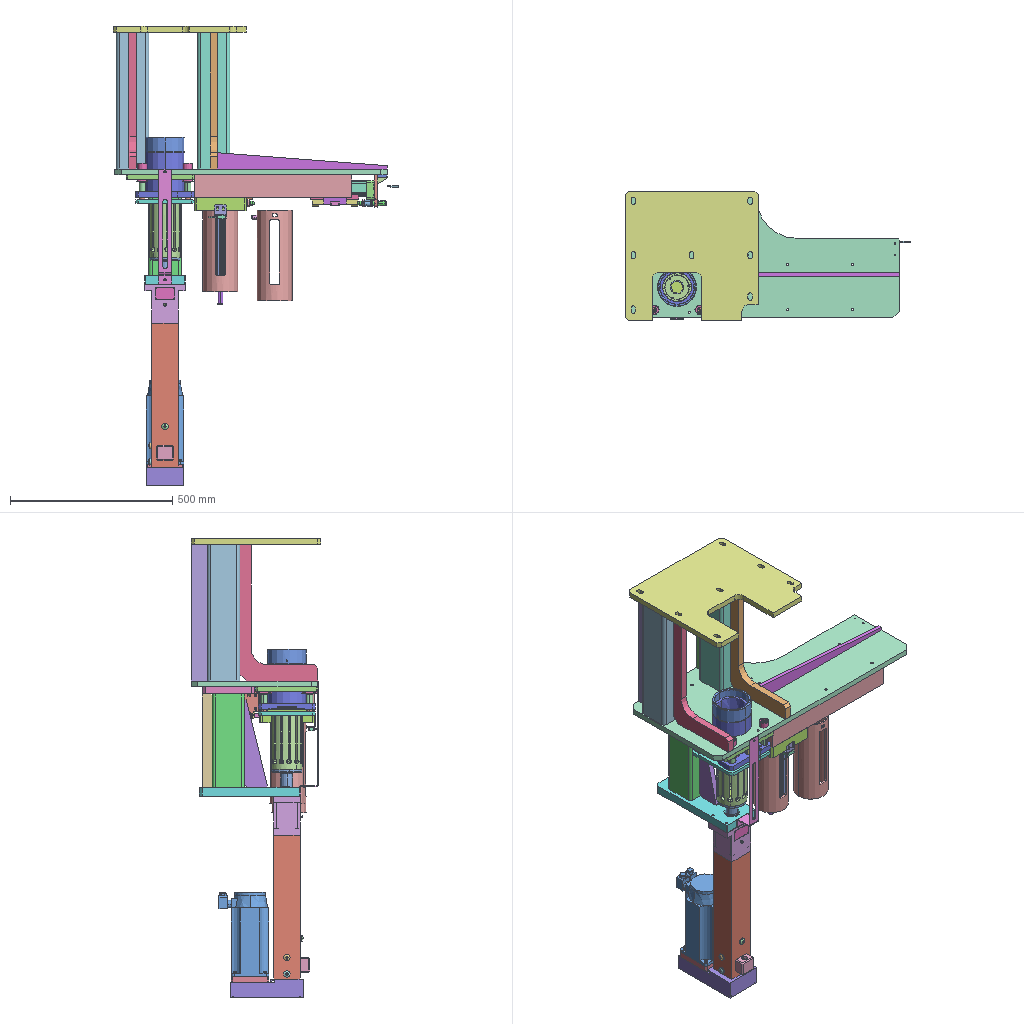Assembly | STEP file | 44 different items | 185 placed | box 880 x 400 x 1414 mm
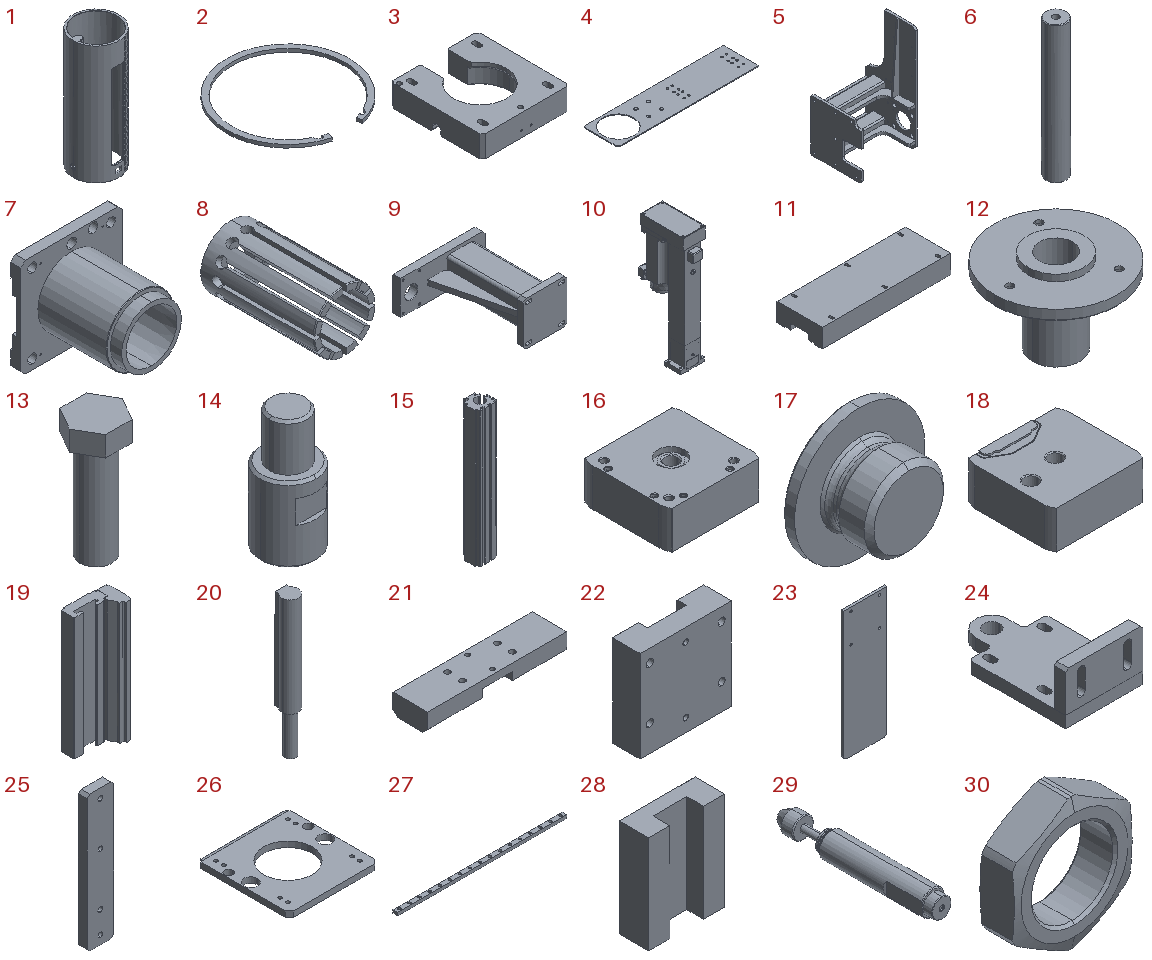Parts list (item | name | quantity | parent item | size | volume):
1 | PN_0010 Magazine clip | x2 | - | 107.5 x 107.5 x 280 mm | 444439 mm3
2 | Snap ring | x112 | in Snap-ring fitting assembly | 96.5 x 95.005 x 2.5 mm | 2880 mm3
3 | PN_0008 Magazine clip fixing seat | x1 | - | 160 x 170 x 40 mm | 624191 mm3
4 | PN_0009 Push plate | x1 | - | 440 x 110 x 10 mm | 235414 mm3
5 | PN_0002 Support seat 2_default_machined_ | x1 | - | 457 x 400 x 845 mm | 11043445 mm3
6 | PN_0006 Pre-compression sleeve guide rod | x4 | - | 16 x 16 x 107 mm | 20796 mm3
7 | PN_0016 Snap-ring guide sleeve | x1 | - | 180 x 160 x 175 mm | 921190 mm3
8 | PN_0005 Press head | x1 | - | 94 x 175 x 94 mm | 368252 mm3
9 | PN_0003 Load-bearing support rod_default_machined_ | x1 | - | 310 x 337 x 160 mm | 2390981 mm3
10 | NP-80-020-300-150V3 (excluding W400-NCFK) Wildermann servo press | x1 | - | - | -
11 | PN_0007 Fixing plate | x1 | - | 484 x 170 x 70 mm | 4861056 mm3
12 | PN_0026 Snap-ring connector | x1 | - | 93 x 93 x 63 mm | 79836 mm3
13 | PN_0027 Punch screw rod | x1 | - | 39.26 x 34 x 90 mm | 48946 mm3
14 | PN_0019 Locating pin | x2 | - | 12 x 12 x 26 mm | 2255 mm3
15 | DGC-25 cylinder body_DGC-25-200-G-PPV-A | x1 | in DGC-25 rodless cylinder_DGC_25_200_G_PPV_A | 52.1 x 48.5 x 351 mm | 492103 mm3
16 | DGC-25-G left fixed end | x1 | in DGC-25 rodless cylinder_DGC_25_200_G_PPV_A | 59.8 x 56.5 x 25.5 mm | 77572 mm3
17 | DGC-25 screw | x4 | in DGC-25 rodless cylinder_DGC_25_200_G_PPV_A | 16 x 7.5 x 16 mm | 612.752 mm3
18 | DGC-25-G right fixed end | x1 | in DGC-25 rodless cylinder_DGC_25_200_G_PPV_A | 59.8 x 56.5 x 25.5 mm | 73184 mm3
19 | DGC-25-G slider | x1 | in DGC-25 rodless cylinder_DGC_25_200_G_PPV_A | 56 x 31.65 x 148 mm | 138361 mm3
20 | SME-8-FM-ZS-24V-K-2.5 0-1E magnetic switch | x2 | in DGC-25 rodless cylinder_DGC_25_200_G_PPV_A | 4 x 4.5 x 34.5 mm | 407.204 mm3
21 | PN_0024 Rodless cylinder connecting plate | x1 | - | 140 x 35 x 20 mm | 68524 mm3
22 | PN_0020 Connecting plate | x1 | - | 70 x 22 x 70 mm | 86429 mm3
23 | PN_0021 Support plate | x1 | - | 60 x 3.8 x 180 mm | 40869 mm3
24 | PN_0022 Rodless cylinder support plate_default_machined_ | x2 | - | 60 x 100 x 40 mm | 60028 mm3
25 | PN_0023 Connecting block | x1 | - | 30 x 10 x 155 mm | 44164 mm3
26 | PN_0025 Snap-ring height stop block | x1 | - | 175 x 180 x 11 mm | 245670 mm3
27 | BMC12B guide rail_L70 | x2 | in BMC12B2NZ1L420II linear guide | 420 x 12 x 7.5 mm | 35533 mm3
28 | BMC12B slider | x4 | in BMC12B2NZ1L420II linear guide | 27 x 11.5 x 34.8 mm | 8068 mm3
29 | ACA-1412 buffer body | x2 | in ACA-1412 hydraulic buffer_ACA-1412-1-P | 14 x 90 x 14 mm | 10668 mm3
30 | ACA-1412 buffer nut | x4 | in ACA-1412 hydraulic buffer_ACA-1412-1-P | 19 x 6 x 21.289 mm | 1012 mm3
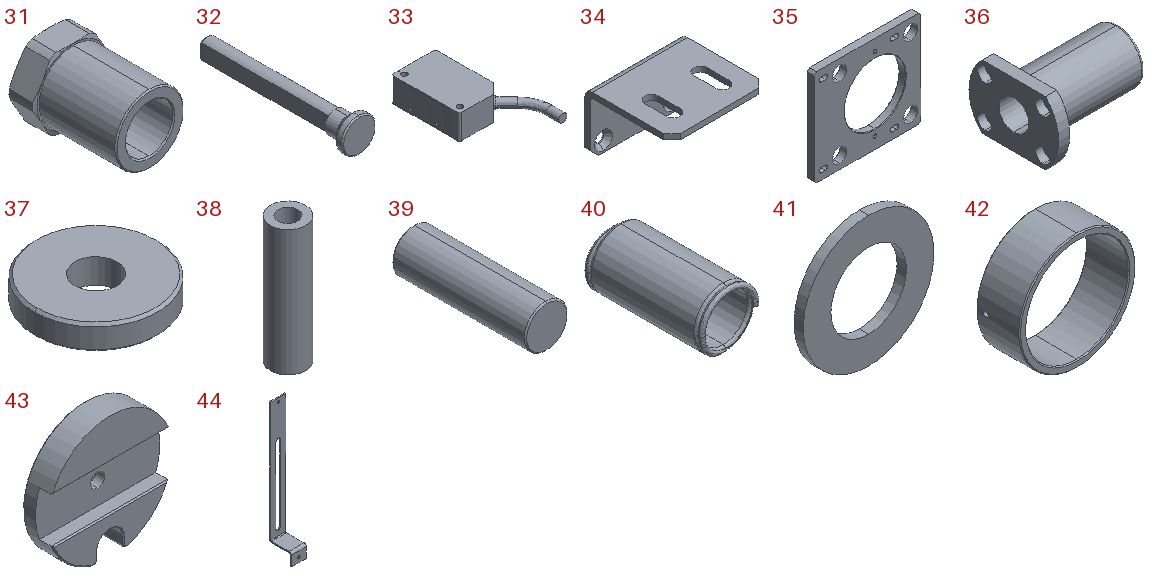31 | F_ACA_LM locating stop nut_F-ACA14-LM | x2 | - | 20.9 x 27 x 19 mm | 3920 mm3
32 | PN_0017 Snap-ring stop plate | x1 | - | 28 x 126.5 x 28 mm | 23542 mm3
33 | CX-441 reflective photoelectric sensor 2--50mm_reflective photoelectric sensor441 | x1 | - | 29.642 x 52.805 x 11.2 mm | 7049 mm3
34 | PN_0018 Sensor bracket | x1 | - | 35 x 32 x 22 mm | 3241 mm3
35 | PN_0015 Pre-compression sleeve guide seat | x1 | - | 210 x 14 x 190 mm | 352968 mm3
36 | LHFCD16 flanged linear bearing_LHFCD16 | x4 | - | 56 x 48 x 34 mm | 27480 mm3
37 | PN_0013 Press plate | x2 | - | 25 x 25 x 5 mm | 2151 mm3
38 | PN_0014 Height locating sleeve | x2 | - | 16 x 16 x 57 mm | 7834 mm3
39 | PN_0011 Handle | x1 | - | 16 x 50 x 16 mm | 9697 mm3
40 | UL20_40 round-wire coil spring_UL20-40 | x4 | - | 20 x 40 x 20 mm | 3902 mm3
41 | PN_0004 Spring seat | x4 | - | 28 x 2 x 28 mm | 819.265 mm3
42 | PN_0001 Snap-ring locating sleeve (for centring) | x1 | - | 120 x 45 x 120 mm | 110978 mm3
43 | PN_0012 Counterweight block | x1 | - | 97 x 20 x 95.103 mm | 106377 mm3
44 | PN_0028 Sensor switch bracket | x1 | - | 40 x 58 x 355 mm | 40391 mm3
Placements (level | parent | child | x y z in mm | rotation matrix by rows):
1 | subassembly 2 | PN_0010 Magazine clip | 83.527 -96.424 311.913 | 1 0 0 0 -1 0 0 0 -1
1 | subassembly 2 | Snap-ring fitting assembly | 16.972 -109.722 137.712 | -0.04372 0.999 0 0.999 0.04372 0 0 0 -1
2 | Snap-ring fitting assembly | Snap ring | 10.376 67.072 87.699 | 1 0 0 0 1 0 0 0 1
2 | Snap-ring fitting assembly | Snap ring | 10.376 67.072 85.199 | 1 0 0 0 1 0 0 0 1
2 | Snap-ring fitting assembly | Snap ring | 10.376 67.072 82.699 | 1 0 0 0 1 0 0 0 1
2 | Snap-ring fitting assembly | Snap ring | 10.376 67.072 80.199 | 1 0 0 0 1 0 0 0 1
2 | Snap-ring fitting assembly | Snap ring | 10.376 67.072 77.699 | 1 0 0 0 1 0 0 0 1
2 | Snap-ring fitting assembly | Snap ring | 10.376 67.072 75.199 | 1 0 0 0 1 0 0 0 1
2 | Snap-ring fitting assembly | Snap ring | 10.376 67.072 72.699 | 1 0 0 0 1 0 0 0 1
2 | Snap-ring fitting assembly | Snap ring | 10.376 67.072 70.199 | 1 0 0 0 1 0 0 0 1
2 | Snap-ring fitting assembly | Snap ring | 10.376 67.072 67.699 | 1 0 0 0 1 0 0 0 1
2 | Snap-ring fitting assembly | Snap ring | 10.376 67.072 65.199 | 1 0 0 0 1 0 0 0 1
2 | Snap-ring fitting assembly | Snap ring | 10.376 67.072 62.699 | 1 0 0 0 1 0 0 0 1
2 | Snap-ring fitting assembly | Snap ring | 10.376 67.072 60.199 | 1 0 0 0 1 0 0 0 1
2 | Snap-ring fitting assembly | Snap ring | 10.376 67.072 57.699 | 1 0 0 0 1 0 0 0 1
2 | Snap-ring fitting assembly | Snap ring | 10.376 67.072 55.199 | 1 0 0 0 1 0 0 0 1
2 | Snap-ring fitting assembly | Snap ring | 10.376 67.072 52.699 | 1 0 0 0 1 0 0 0 1
2 | Snap-ring fitting assembly | Snap ring | 10.376 67.072 50.199 | 1 0 0 0 1 0 0 0 1
2 | Snap-ring fitting assembly | Snap ring | 10.376 67.072 47.699 | 1 0 0 0 1 0 0 0 1
2 | Snap-ring fitting assembly | Snap ring | 10.376 67.072 45.199 | 1 0 0 0 1 0 0 0 1
2 | Snap-ring fitting assembly | Snap ring | 10.376 67.072 42.699 | 1 0 0 0 1 0 0 0 1
2 | Snap-ring fitting assembly | Snap ring | 10.376 67.072 40.199 | 1 0 0 0 1 0 0 0 1
2 | Snap-ring fitting assembly | Snap ring | 10.376 67.072 37.699 | 1 0 0 0 1 0 0 0 1
2 | Snap-ring fitting assembly | Snap ring | 10.376 67.072 35.199 | 1 0 0 0 1 0 0 0 1
2 | Snap-ring fitting assembly | Snap ring | 10.376 67.072 32.699 | 1 0 0 0 1 0 0 0 1
2 | Snap-ring fitting assembly | Snap ring | 10.376 67.072 30.199 | 1 0 0 0 1 0 0 0 1
2 | Snap-ring fitting assembly | Snap ring | 10.376 67.072 27.699 | 1 0 0 0 1 0 0 0 1
2 | Snap-ring fitting assembly | Snap ring | 10.376 67.072 25.199 | 1 0 0 0 1 0 0 0 1
2 | Snap-ring fitting assembly | Snap ring | 10.376 67.072 22.699 | 1 0 0 0 1 0 0 0 1
2 | Snap-ring fitting assembly | Snap ring | 10.376 67.072 20.199 | 1 0 0 0 1 0 0 0 1
2 | Snap-ring fitting assembly | Snap ring | 10.376 67.072 17.699 | 1 0 0 0 1 0 0 0 1
2 | Snap-ring fitting assembly | Snap ring | 10.376 67.072 15.199 | 1 0 0 0 1 0 0 0 1
2 | Snap-ring fitting assembly | Snap ring | 10.376 67.072 12.699 | 1 0 0 0 1 0 0 0 1
2 | Snap-ring fitting assembly | Snap ring | 10.376 67.072 10.199 | 1 0 0 0 1 0 0 0 1
2 | Snap-ring fitting assembly | Snap ring | 10.376 67.072 7.699 | 1 0 0 0 1 0 0 0 1
2 | Snap-ring fitting assembly | Snap ring | 10.376 67.072 5.199 | 1 0 0 0 1 0 0 0 1
2 | Snap-ring fitting assembly | Snap ring | 10.376 67.072 2.699 | 1 0 0 0 1 0 0 0 1
2 | Snap-ring fitting assembly | Snap ring | 10.376 67.072 0.1993 | 1 0 0 0 1 0 0 0 1
2 | Snap-ring fitting assembly | Snap ring | 10.376 67.072 -2.301 | 1 0 0 0 1 0 0 0 1
2 | Snap-ring fitting assembly | Snap ring | 10.376 67.072 -4.801 | 1 0 0 0 1 0 0 0 1
2 | Snap-ring fitting assembly | Snap ring | 10.376 67.072 -7.301 | 1 0 0 0 1 0 0 0 1
2 | Snap-ring fitting assembly | Snap ring | 10.376 67.072 -9.801 | 1 0 0 0 1 0 0 0 1
2 | Snap-ring fitting assembly | Snap ring | 10.376 67.072 -12.301 | 1 0 0 0 1 0 0 0 1
2 | Snap-ring fitting assembly | Snap ring | 10.376 67.072 -14.801 | 1 0 0 0 1 0 0 0 1
2 | Snap-ring fitting assembly | Snap ring | 10.376 67.072 -17.301 | 1 0 0 0 1 0 0 0 1
2 | Snap-ring fitting assembly | Snap ring | 10.376 67.072 -19.801 | 1 0 0 0 1 0 0 0 1
2 | Snap-ring fitting assembly | Snap ring | 10.376 67.072 -22.301 | 1 0 0 0 1 0 0 0 1
2 | Snap-ring fitting assembly | Snap ring | 10.376 67.072 -24.801 | 1 0 0 0 1 0 0 0 1
2 | Snap-ring fitting assembly | Snap ring | 10.376 67.072 -27.301 | 1 0 0 0 1 0 0 0 1
2 | Snap-ring fitting assembly | Snap ring | 10.376 67.072 -29.801 | 1 0 0 0 1 0 0 0 1
2 | Snap-ring fitting assembly | Snap ring | 10.376 67.072 -32.301 | 1 0 0 0 1 0 0 0 1
2 | Snap-ring fitting assembly | Snap ring | 10.376 67.072 -34.801 | 1 0 0 0 1 0 0 0 1
2 | Snap-ring fitting assembly | Snap ring | 10.376 67.072 -37.301 | 1 0 0 0 1 0 0 0 1
2 | Snap-ring fitting assembly | Snap ring | 10.376 67.072 -39.801 | 1 0 0 0 1 0 0 0 1
2 | Snap-ring fitting assembly | Snap ring | 10.376 67.072 -42.301 | 1 0 0 0 1 0 0 0 1
2 | Snap-ring fitting assembly | Snap ring | 10.376 67.072 -44.801 | 1 0 0 0 1 0 0 0 1
2 | Snap-ring fitting assembly | Snap ring | 10.376 67.072 -47.301 | 1 0 0 0 1 0 0 0 1
2 | Snap-ring fitting assembly | Snap ring | 10.376 67.072 -49.801 | 1 0 0 0 1 0 0 0 1
2 | Snap-ring fitting assembly | Snap ring | 10.376 67.072 -52.301 | 1 0 0 0 1 0 0 0 1
2 | Snap-ring fitting assembly | Snap ring | 10.376 67.072 -54.801 | 1 0 0 0 1 0 0 0 1
2 | Snap-ring fitting assembly | Snap ring | 10.376 67.072 -57.301 | 1 0 0 0 1 0 0 0 1
2 | Snap-ring fitting assembly | Snap ring | 10.376 67.072 -59.801 | 1 0 0 0 1 0 0 0 1
2 | Snap-ring fitting assembly | Snap ring | 10.376 67.072 -62.301 | 1 0 0 0 1 0 0 0 1
2 | Snap-ring fitting assembly | Snap ring | 10.376 67.072 -64.801 | 1 0 0 0 1 0 0 0 1
2 | Snap-ring fitting assembly | Snap ring | 10.376 67.072 -67.301 | 1 0 0 0 1 0 0 0 1
2 | Snap-ring fitting assembly | Snap ring | 10.376 67.072 -69.801 | 1 0 0 0 1 0 0 0 1
2 | Snap-ring fitting assembly | Snap ring | 10.376 67.072 -72.301 | 1 0 0 0 1 0 0 0 1
2 | Snap-ring fitting assembly | Snap ring | 10.376 67.072 -74.801 | 1 0 0 0 1 0 0 0 1
2 | Snap-ring fitting assembly | Snap ring | 10.376 67.072 -77.301 | 1 0 0 0 1 0 0 0 1
2 | Snap-ring fitting assembly | Snap ring | 10.376 67.072 -79.801 | 1 0 0 0 1 0 0 0 1
2 | Snap-ring fitting assembly | Snap ring | 10.376 67.072 -82.301 | 1 0 0 0 1 0 0 0 1
2 | Snap-ring fitting assembly | Snap ring | 10.376 67.072 -84.801 | 1 0 0 0 1 0 0 0 1
2 | Snap-ring fitting assembly | Snap ring | 10.376 67.072 -87.301 | 1 0 0 0 1 0 0 0 1
2 | Snap-ring fitting assembly | Snap ring | 10.376 67.072 -89.801 | 1 0 0 0 1 0 0 0 1
2 | Snap-ring fitting assembly | Snap ring | 10.376 67.072 -92.301 | 1 0 0 0 1 0 0 0 1
2 | Snap-ring fitting assembly | Snap ring | 10.376 67.072 -94.801 | 1 0 0 0 1 0 0 0 1
2 | Snap-ring fitting assembly | Snap ring | 10.376 67.072 -97.301 | 1 0 0 0 1 0 0 0 1
2 | Snap-ring fitting assembly | Snap ring | 10.376 67.072 -99.801 | 1 0 0 0 1 0 0 0 1
2 | Snap-ring fitting assembly | Snap ring | 10.376 67.072 -102.301 | 1 0 0 0 1 0 0 0 1
2 | Snap-ring fitting assembly | Snap ring | 10.376 67.072 -104.801 | 1 0 0 0 1 0 0 0 1
2 | Snap-ring fitting assembly | Snap ring | 10.376 67.072 -107.301 | 1 0 0 0 1 0 0 0 1
2 | Snap-ring fitting assembly | Snap ring | 10.376 67.072 -109.801 | 1 0 0 0 1 0 0 0 1
2 | Snap-ring fitting assembly | Snap ring | 10.376 67.072 -112.301 | 1 0 0 0 1 0 0 0 1
2 | Snap-ring fitting assembly | Snap ring | 10.376 67.072 -114.801 | 1 0 0 0 1 0 0 0 1
2 | Snap-ring fitting assembly | Snap ring | 10.376 67.072 -117.301 | 1 0 0 0 1 0 0 0 1
2 | Snap-ring fitting assembly | Snap ring | 10.376 67.072 -119.801 | 1 0 0 0 1 0 0 0 1
2 | Snap-ring fitting assembly | Snap ring | 10.376 67.072 -122.301 | 1 0 0 0 1 0 0 0 1
2 | Snap-ring fitting assembly | Snap ring | 10.376 67.072 -124.801 | 1 0 0 0 1 0 0 0 1
2 | Snap-ring fitting assembly | Snap ring | 10.376 67.072 -127.301 | 1 0 0 0 1 0 0 0 1
2 | Snap-ring fitting assembly | Snap ring | 10.376 67.072 -129.801 | 1 0 0 0 1 0 0 0 1
2 | Snap-ring fitting assembly | Snap ring | 10.376 67.072 -132.301 | 1 0 0 0 1 0 0 0 1
2 | Snap-ring fitting assembly | Snap ring | 10.376 67.072 -134.801 | 1 0 0 0 1 0 0 0 1
2 | Snap-ring fitting assembly | Snap ring | 10.376 67.072 -137.301 | 1 0 0 0 1 0 0 0 1
2 | Snap-ring fitting assembly | Snap ring | 10.376 67.072 -139.801 | 1 0 0 0 1 0 0 0 1
2 | Snap-ring fitting assembly | Snap ring | 10.376 67.072 -142.301 | 1 0 0 0 1 0 0 0 1
2 | Snap-ring fitting assembly | Snap ring | 10.376 67.072 -144.801 | 1 0 0 0 1 0 0 0 1
2 | Snap-ring fitting assembly | Snap ring | 10.376 67.072 -147.301 | 1 0 0 0 1 0 0 0 1
2 | Snap-ring fitting assembly | Snap ring | 10.376 67.072 -149.801 | 1 0 0 0 1 0 0 0 1
2 | Snap-ring fitting assembly | Snap ring | 10.376 67.072 -152.301 | 1 0 0 0 1 0 0 0 1
2 | Snap-ring fitting assembly | Snap ring | 10.376 67.072 -154.801 | 1 0 0 0 1 0 0 0 1
2 | Snap-ring fitting assembly | Snap ring | 10.376 67.072 -157.301 | 1 0 0 0 1 0 0 0 1
2 | Snap-ring fitting assembly | Snap ring | 10.376 67.072 -159.801 | 1 0 0 0 1 0 0 0 1
2 | Snap-ring fitting assembly | Snap ring | 10.376 67.072 -162.301 | 1 0 0 0 1 0 0 0 1
2 | Snap-ring fitting assembly | Snap ring | 10.376 67.072 -164.801 | 1 0 0 0 1 0 0 0 1
2 | Snap-ring fitting assembly | Snap ring | 10.376 67.072 -167.301 | 1 0 0 0 1 0 0 0 1
2 | Snap-ring fitting assembly | Snap ring | 10.376 67.072 -169.801 | 1 0 0 0 1 0 0 0 1
2 | Snap-ring fitting assembly | Snap ring | 10.376 67.072 -172.301 | 1 0 0 0 1 0 0 0 1
2 | Snap-ring fitting assembly | Snap ring | 10.376 67.072 -174.801 | 1 0 0 0 1 0 0 0 1
2 | Snap-ring fitting assembly | Snap ring | 10.376 67.072 -177.301 | 1 0 0 0 1 0 0 0 1
2 | Snap-ring fitting assembly | Snap ring | 10.376 67.072 -179.801 | 1 0 0 0 1 0 0 0 1
2 | Snap-ring fitting assembly | Snap ring | 10.376 67.072 -182.301 | 1 0 0 0 1 0 0 0 1
2 | Snap-ring fitting assembly | Snap ring | 10.376 67.072 -184.801 | 1 0 0 0 1 0 0 0 1
1 | subassembly 2 | PN_0008 Magazine clip fixing seat | 83.527 -96.424 321.913 | 1 0 0 0 1 0 0 0 1
1 | subassembly 2 | PN_0009 Push plate | 251.549 -96.424 324.913 | 1 0 0 0 -1 0 0 0 -1
1 | subassembly 2 | Snap ring | 83.527 -96.424 322.512 | 0.1475 0.9891 0 -0.9891 0.1475 0 0 0 1
1 | subassembly 2 | PN_0002 Support seat 2_default_machined_ | 63.027 98.576 830.913 | 0 0 1 0 1 0 -1 0 0
1 | subassembly 2 | PN_0006 Pre-compression sleeve guide rod | -156.973 -26.424 421.712 | -0.9255 0.3788 0 0.3788 0.9255 0 0 0 -1
1 | subassembly 2 | PN_0006 Pre-compression sleeve guide rod | -156.973 -166.424 421.712 | 0.9969 0.07931 0 0.07931 -0.9969 0 0 0 -1
1 | subassembly 2 | PN_0006 Pre-compression sleeve guide rod | -16.973 -166.424 421.712 | 0.8302 0.5574 0 0.5574 -0.8302 0 0 0 -1
1 | subassembly 2 | PN_0006 Pre-compression sleeve guide rod | -16.973 -26.424 421.712 | 0 -1 0 -1 0 0 0 0 -1
1 | subassembly 2 | PN_0016 Snap-ring guide sleeve | -86.973 -96.424 492.212 | 1 0 0 0 0 1 0 -1 0
1 | subassembly 2 | PN_0005 Press head | -86.973 -96.424 136.912 | 0.6232 0 0.7821 -0.7821 0 0.6232 0 -1 -0
1 | subassembly 2 | PN_0003 Load-bearing support rod_default_machined_ | -86.973 83.576 81.912 | 0 0 -1 1 0 0 0 -1 0
1 | subassembly 2 | NP-80-020-300-150V3 (excluding W400-NCFK) Wildermann servo press | -86.973 -96.424 -122.088 | -1 -1e-05 0 -1e-05 1 0 0 0 -1
1 | subassembly 2 | PN_0007 Fixing plate | 245.527 -96.424 321.913 | 1 0 0 0 1 0 0 0 1
1 | subassembly 2 | PN_0026 Snap-ring connector | -86.973 -96.424 78.912 | -0.9889 0.1487 0 -0.1487 -0.9889 0 0 0 1
1 | subassembly 2 | PN_0027 Punch screw rod | -86.973 -96.424 66.912 | 0.9798 0.2001 0 -0.2001 0.9798 0 0 0 1
1 | subassembly 2 | PN_0019 Locating pin | 16.777 -96.424 289.913 | 0 0 1 0.6934 0.7205 0 -0.7205 0.6934 0
1 | subassembly 2 | DGC-25 rodless cylinder_DGC_25_200_G_PPV_A | 182.527 22.326 373.413 | 0 0 -1 1 0 0 0 -1 -0
2 | DGC-25 rodless cylinder_DGC_25_200_G_PPV_A | DGC-25 cylinder body_DGC-25-200-G-PPV-A | -0.0 -0.0 -0.0 | 1 0 0 0 1 0 0 0 1
2 | DGC-25 rodless cylinder_DGC_25_200_G_PPV_A | DGC-25-G left fixed end | -0.0 -0.0 24.5 | 1 0 0 0 1 0 0 0 1
2 | DGC-25 rodless cylinder_DGC_25_200_G_PPV_A | DGC-25 screw | 28.4 26.1 14.0 | 0 1 0 0 0 -1 -1 0 -0
2 | DGC-25 rodless cylinder_DGC_25_200_G_PPV_A | DGC-25 screw | 0.1 29.0 23.0 | 1 0 0 0 0 -1 0 1 0
2 | DGC-25 rodless cylinder_DGC_25_200_G_PPV_A | DGC-25-G right fixed end | 0.0 -0.0 -375.5 | 1 0 0 0 1 0 0 0 1
2 | DGC-25 rodless cylinder_DGC_25_200_G_PPV_A | DGC-25 screw | 0.1 29.0 -374.0 | 1 0 0 0 0 1 0 -1 0
2 | DGC-25 rodless cylinder_DGC_25_200_G_PPV_A | DGC-25 screw | -20.6 24.0 -374.0 | 1 0 0 0 0 1 0 -1 0
2 | DGC-25 rodless cylinder_DGC_25_200_G_PPV_A | DGC-25-G slider | 0.0 -0.0 -254.022 | 1 0 0 0 1 0 0 0 1
2 | DGC-25 rodless cylinder_DGC_25_200_G_PPV_A | SME-8-FM-ZS-24V-K-2.5 0-1E magnetic switch | 19.7 17.0 0.0 | 0 1 0 -1 0 0 0 0 1
2 | DGC-25 rodless cylinder_DGC_25_200_G_PPV_A | SME-8-FM-ZS-24V-K-2.5 0-1E magnetic switch | 19.7 17.0 -451.0 | 0 1 0 1 0 0 0 0 -1
1 | subassembly 2 | PN_0024 Rodless cylinder connecting plate | 436.549 2.576 299.913 | 1 0 0 0 1 0 0 0 1
1 | subassembly 2 | PN_0020 Connecting plate | 436.549 -77.424 322.512 | -1 0 0 0 0 -1 0 -1 0
1 | subassembly 2 | PN_0021 Support plate | 116.549 -96.424 331.913 | 0 0 1 -1 0 0 0 -1 0
1 | subassembly 2 | PN_0022 Rodless cylinder support plate_default_machined_ | 158.027 20.076 391.913 | 0 0 -1 1 0 0 0 -1 -0
1 | subassembly 2 | PN_0022 Rodless cylinder support plate_default_machined_ | 558.027 20.076 391.913 | 0 0 1 -1 0 0 0 -1 0
1 | subassembly 2 | PN_0023 Connecting block | 436.549 -34.924 308.413 | -1 0 0 0 0 -1 0 -1 0
1 | subassembly 2 | Snap ring | 86.549 -96.424 324.913 | -0.03942 0.9992 0 0.9992 0.03942 0 0 0 -1
1 | subassembly 2 | PN_0025 Snap-ring height stop block | -86.973 -96.424 303.712 | 0 1 0 -1 0 0 0 0 1
1 | subassembly 2 | BMC12B2NZ1L420II linear guide | 326.793 -143.035 394.18 | -1 0 0 0 1 0 0 0 -1
2 | BMC12B2NZ1L420II linear guide | BMC12B guide rail_L70 | 49.267 62.861 52.418 | 1 0 0 0 1 0 0 0 1
2 | BMC12B2NZ1L420II linear guide | BMC12B slider | 52.745 62.861 50.168 | 0 0 1 1 0 0 0 1 0
2 | BMC12B2NZ1L420II linear guide | BMC12B slider | -117.255 62.861 50.168 | 0 0 1 1 0 0 0 1 0
1 | subassembly 2 | BMC12B2NZ1L420II linear guide | 326.793 -175.535 394.18 | -1 0 0 0 1 0 0 0 -1
2 | BMC12B2NZ1L420II linear guide | BMC12B guide rail_L70 | 49.267 62.861 52.418 | 1 0 0 0 1 0 0 0 1
2 | BMC12B2NZ1L420II linear guide | BMC12B slider | 52.745 62.861 50.168 | 0 0 1 1 0 0 0 1 0
2 | BMC12B2NZ1L420II linear guide | BMC12B slider | -117.255 62.861 50.168 | 0 0 1 1 0 0 0 1 0
1 | subassembly 2 | ACA-1412 hydraulic buffer_ACA-1412-1-P | 596.449 20.076 304.413 | 0 -1 0 0.9634 0 0.2679 -0.2679 0 0.9634
2 | ACA-1412 hydraulic buffer_ACA-1412-1-P | ACA-1412 buffer body | -0.0 -0.0 -0.0 | 1 0 0 0 1 0 0 0 1
2 | ACA-1412 hydraulic buffer_ACA-1412-1-P | ACA-1412 buffer nut | -0.0 69.588 -0.0 | 1 0 0 0 1 0 0 0 1
2 | ACA-1412 hydraulic buffer_ACA-1412-1-P | ACA-1412 buffer nut | -0.0 45.424 -0.0 | 1 0 0 0 1 0 0 0 1
1 | subassembly 2 | F_ACA_LM locating stop nut_F-ACA14-LM | 525.027 20.076 304.413 | 0 1 0 0.4997 0 0.8662 0.8662 0 -0.4997
1 | subassembly 2 | ACA-1412 hydraulic buffer_ACA-1412-1-P | 97.603 20.076 304.413 | 0 1 0 -0.4763 0 0.8793 0.8793 0 0.4763
2 | ACA-1412 hydraulic buffer_ACA-1412-1-P | ACA-1412 buffer body | -0.0 -0.0 -0.0 | 1 0 0 0 1 0 0 0 1
2 | ACA-1412 hydraulic buffer_ACA-1412-1-P | ACA-1412 buffer nut | -0.0 69.588 -0.0 | 1 0 0 0 1 0 0 0 1
2 | ACA-1412 hydraulic buffer_ACA-1412-1-P | ACA-1412 buffer nut | -0.0 45.424 -0.0 | 1 0 0 0 1 0 0 0 1
1 | subassembly 2 | F_ACA_LM locating stop nut_F-ACA14-LM | 159.356 20.076 304.413 | 0 -1 0 0.9631 0 0.2691 -0.2691 0 0.9631
1 | subassembly 2 | PN_0017 Snap-ring stop plate | 83.527 -42.674 295.913 | 0 0 1 0 -1 0 1 0 0
1 | subassembly 2 | CX-441 reflective photoelectric sensor 2--50mm_reflective photoelectric sensor441 | 83.527 -162.424 261.65 | 0 1 0 -1 0 0 0 0 1
1 | subassembly 2 | PN_0018 Sensor bracket | 83.527 -171.424 267.25 | -1 0 0 0 0 -1 0 -1 -0
1 | subassembly 2 | PN_0015 Pre-compression sleeve guide seat | -86.973 -96.424 391.913 | 1 0 0 0 0 1 0 -1 0
1 | subassembly 2 | LHFCD16 flanged linear bearing_LHFCD16 | -156.973 -166.424 371.913 | 0 0 -1 0 1 0 1 0 -0
1 | subassembly 2 | LHFCD16 flanged linear bearing_LHFCD16 | -16.973 -166.424 371.913 | 0 0 1 0 -1 0 1 0 -0
1 | subassembly 2 | LHFCD16 flanged linear bearing_LHFCD16 | -16.973 -26.424 371.913 | 0 0 1 0 -1 0 1 0 0
1 | subassembly 2 | LHFCD16 flanged linear bearing_LHFCD16 | -156.973 -26.424 371.913 | 0 0 -1 0 1 0 1 0 -0
1 | subassembly 2 | PN_0013 Press plate | -86.973 -168.924 315.913 | 1 0 0 0 1 0 0 0 1
1 | subassembly 2 | PN_0014 Height locating sleeve | -86.973 -168.924 320.913 | 0.9986 -0.05244 0 0.05244 0.9986 0 0 0 1
1 | subassembly 2 | PN_0014 Height locating sleeve | -86.973 -23.924 320.913 | 1 0 0 0 1 0 0 0 1
1 | subassembly 2 | PN_0013 Press plate | -86.973 -23.924 315.913 | 1 0 0 0 1 0 0 0 1
1 | subassembly 2 | PN_0011 Handle | 83.527 -96.424 -6.29 | 1 0 0 0 0 -1 0 1 -0
1 | subassembly 2 | UL20_40 round-wire coil spring_UL20-40 | -16.973 -166.424 351.712 | 1 0 0 0 0 1 0 -1 0
1 | subassembly 2 | PN_0004 Spring seat | -16.973 -166.424 371.913 | 1 0 0 0 0 1 0 -1 0
1 | subassembly 2 | PN_0004 Spring seat | -16.973 -26.424 371.913 | 0 0 -1 1 0 0 0 -1 -0
1 | subassembly 2 | PN_0004 Spring seat | -156.973 -26.424 371.913 | -1 0 0 0 0 -1 0 -1 -0
1 | subassembly 2 | PN_0004 Spring seat | -156.973 -166.424 371.913 | 0 0 1 -1 0 0 0 -1 0
1 | subassembly 2 | UL20_40 round-wire coil spring_UL20-40 | -16.973 -26.424 351.712 | 0 0 -1 1 0 0 0 -1 0
1 | subassembly 2 | UL20_40 round-wire coil spring_UL20-40 | -156.973 -26.424 351.712 | -1 0 0 0 0 -1 0 -1 0
1 | subassembly 2 | UL20_40 round-wire coil spring_UL20-40 | -156.973 -166.424 351.712 | 0 0 1 -1 0 0 0 -1 0
1 | subassembly 2 | PN_0001 Snap-ring locating sleeve (for centring) | -86.973 -96.424 507.212 | 1 0 0 0 0 1 0 -1 0
1 | subassembly 2 | PN_0010 Magazine clip | 250.613 -103.148 283.393 | 1 0 0 0 -1 0 0 0 -1
1 | subassembly 2 | PN_0012 Counterweight block | 83.527 -96.424 63.71 | -0.03666 0 0.9993 -0.9993 0 -0.03666 0 -1 -0
1 | subassembly 2 | PN_0028 Sensor switch bracket | -86.973 -191.424 248.912 | -1 0 0 0 -1 0 0 0 1
1 | subassembly 2 | PN_0019 Locating pin | 180.863 -103.148 261.393 | 0 0 1 0.6934 0.7205 0 -0.7205 0.6934 0